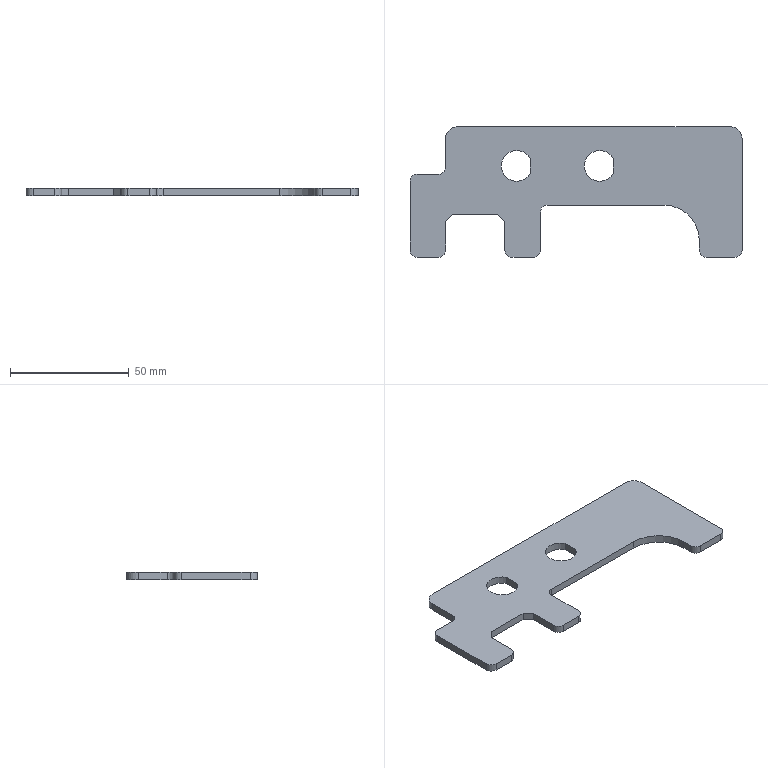Part | SolidWorks | features FlatPattern 1, SMBaseFlange 1, SheetMetal 1 | 1 solid | 36 faces | box 140 x 55 x 3.2 mm | volume 16813 mm3 | plane 20 | cylinder 16 | commonest cylinder face diameters 6 x9 13 x4 10 x2 30 x1
STEP:
#1=CARTESIAN_POINT('',(-66.3,99.624,3.2));
#2=VERTEX_POINT('',#1);
#3=CARTESIAN_POINT('',(-78.5,96.5,3.2));
#4=VERTEX_POINT('',#3);
#5=CARTESIAN_POINT('',(-72.,96.5,3.2));
#6=DIRECTION('',(0.,0.,1.));
#7=DIRECTION('',(1.,0.,0.));
#8=AXIS2_PLACEMENT_3D('',#5,#6,#7);
#9=CIRCLE('',#8,6.5);
#10=EDGE_CURVE('',#2,#4,#9,.T.);
#11=ORIENTED_EDGE('',*,*,#10,.T.);
#12=CARTESIAN_POINT('',(-78.5,96.5,0.));
#13=VERTEX_POINT('',#12);
#14=CARTESIAN_POINT('',(-78.5,96.5,3.2));
#15=DIRECTION('',(0.,0.,-1.));
#16=VECTOR('',#15,1000.);
#17=LINE('',#14,#16);
#18=EDGE_CURVE('',#4,#13,#17,.T.);
#19=ORIENTED_EDGE('',*,*,#18,.T.);
#20=CARTESIAN_POINT('',(-66.3,99.624,0.));
#21=VERTEX_POINT('',#20);
#22=CARTESIAN_POINT('',(-72.,96.5,0.));
#23=DIRECTION('',(0.,0.,1.));
#24=DIRECTION('',(1.,0.,0.));
#25=AXIS2_PLACEMENT_3D('',#22,#23,#24);
#26=CIRCLE('',#25,6.5);
#27=EDGE_CURVE('',#21,#13,#26,.T.);
#28=ORIENTED_EDGE('',*,*,#27,.F.);
#29=CARTESIAN_POINT('',(-66.3,99.624,3.2));
#30=DIRECTION('',(0.,0.,-1.));
#31=VECTOR('',#30,1000.);
#32=LINE('',#29,#31);
#33=EDGE_CURVE('',#2,#21,#32,.T.);
#34=ORIENTED_EDGE('',*,*,#33,.F.);
#35=EDGE_LOOP('',(#11,#19,#28,#34));
#36=FACE_OUTER_BOUND('',#35,.T.);
#37=CARTESIAN_POINT('',(-72.,96.5,3.2));
#38=DIRECTION('',(0.,0.,-1.));
#39=DIRECTION('',(-1.,0.,0.));
#40=AXIS2_PLACEMENT_3D('',#37,#38,#39);
#41=CYLINDRICAL_SURFACE('',#40,6.5);
#42=ADVANCED_FACE('',(#36),#41,.F.);
#43=CARTESIAN_POINT('',(-101.3,99.624,3.2));
#44=VERTEX_POINT('',#43);
#45=CARTESIAN_POINT('',(-113.5,96.5,3.2));
#46=VERTEX_POINT('',#45);
#47=CARTESIAN_POINT('',(-107.,96.5,3.2));
#48=DIRECTION('',(0.,0.,1.));
#49=DIRECTION('',(1.,0.,0.));
#50=AXIS2_PLACEMENT_3D('',#47,#48,#49);
#51=CIRCLE('',#50,6.5);
#52=EDGE_CURVE('',#44,#46,#51,.T.);
#53=ORIENTED_EDGE('',*,*,#52,.T.);
#54=CARTESIAN_POINT('',(-113.5,96.5,0.));
#55=VERTEX_POINT('',#54);
#56=CARTESIAN_POINT('',(-113.5,96.5,3.2));
#57=DIRECTION('',(0.,0.,-1.));
#58=VECTOR('',#57,1000.);
#59=LINE('',#56,#58);
#60=EDGE_CURVE('',#46,#55,#59,.T.);
#61=ORIENTED_EDGE('',*,*,#60,.T.);
#62=CARTESIAN_POINT('',(-101.3,99.624,0.));
#63=VERTEX_POINT('',#62);
#64=CARTESIAN_POINT('',(-107.,96.5,0.));
#65=DIRECTION('',(0.,0.,1.));
#66=DIRECTION('',(1.,0.,0.));
#67=AXIS2_PLACEMENT_3D('',#64,#65,#66);
#68=CIRCLE('',#67,6.5);
#69=EDGE_CURVE('',#63,#55,#68,.T.);
#70=ORIENTED_EDGE('',*,*,#69,.F.);
#71=CARTESIAN_POINT('',(-101.3,99.624,3.2));
#72=DIRECTION('',(0.,0.,-1.));
#73=VECTOR('',#72,1000.);
#74=LINE('',#71,#73);
#75=EDGE_CURVE('',#44,#63,#74,.T.);
#76=ORIENTED_EDGE('',*,*,#75,.F.);
#77=EDGE_LOOP('',(#53,#61,#70,#76));
#78=FACE_OUTER_BOUND('',#77,.T.);
#79=CARTESIAN_POINT('',(-107.,96.5,3.2));
#80=DIRECTION('',(0.,0.,-1.));
#81=DIRECTION('',(-1.,0.,0.));
#82=AXIS2_PLACEMENT_3D('',#79,#80,#81);
#83=CYLINDRICAL_SURFACE('',#82,6.5);
#84=ADVANCED_FACE('',(#78),#83,.F.);
#85=ORIENTED_EDGE('',*,*,#52,.F.);
#86=CARTESIAN_POINT('',(-101.3,93.376,3.2));
#87=VERTEX_POINT('',#86);
#88=CARTESIAN_POINT('',(-101.3,93.376,3.2));
#89=DIRECTION('',(0.,1.,0.));
#90=VECTOR('',#89,1000.);
#91=LINE('',#88,#90);
#92=EDGE_CURVE('',#87,#44,#91,.T.);
#93=ORIENTED_EDGE('',*,*,#92,.F.);
#94=CARTESIAN_POINT('',(-107.,96.5,3.2));
#95=DIRECTION('',(0.,0.,1.));
#96=DIRECTION('',(1.,0.,0.));
#97=AXIS2_PLACEMENT_3D('',#94,#95,#96);
#98=CIRCLE('',#97,6.5);
#99=EDGE_CURVE('',#46,#87,#98,.T.);
#100=ORIENTED_EDGE('',*,*,#99,.F.);
#101=EDGE_LOOP('',(#85,#93,#100));
#102=FACE_BOUND('',#101,.T.);
#103=CARTESIAN_POINT('',(-137.,96.,3.2));
#104=VERTEX_POINT('',#103);
#105=CARTESIAN_POINT('',(-140.,93.,3.2));
#106=VERTEX_POINT('',#105);
#107=CARTESIAN_POINT('',(-140.,96.,3.2));
#108=DIRECTION('',(0.,0.,-1.));
#109=DIRECTION('',(-1.,0.,0.));
#110=AXIS2_PLACEMENT_3D('',#107,#108,#109);
#111=CIRCLE('',#110,3.);
#112=EDGE_CURVE('',#104,#106,#111,.T.);
#113=ORIENTED_EDGE('',*,*,#112,.T.);
#114=CARTESIAN_POINT('',(-149.,93.,3.2));
#115=VERTEX_POINT('',#114);
#116=CARTESIAN_POINT('',(-140.,93.,3.2));
#117=DIRECTION('',(-1.,0.,0.));
#118=VECTOR('',#117,1000.);
#119=LINE('',#116,#118);
#120=EDGE_CURVE('',#106,#115,#119,.T.);
#121=ORIENTED_EDGE('',*,*,#120,.T.);
#122=CARTESIAN_POINT('',(-152.,90.,3.2));
#123=VERTEX_POINT('',#122);
#124=CARTESIAN_POINT('',(-149.,90.,3.2));
#125=DIRECTION('',(0.,0.,1.));
#126=DIRECTION('',(1.,0.,0.));
#127=AXIS2_PLACEMENT_3D('',#124,#125,#126);
#128=CIRCLE('',#127,3.);
#129=EDGE_CURVE('',#115,#123,#128,.T.);
#130=ORIENTED_EDGE('',*,*,#129,.T.);
#131=CARTESIAN_POINT('',(-152.,61.,3.2));
#132=VERTEX_POINT('',#131);
#133=CARTESIAN_POINT('',(-152.,90.,3.2));
#134=DIRECTION('',(0.,-1.,0.));
#135=VECTOR('',#134,1000.);
#136=LINE('',#133,#135);
#137=EDGE_CURVE('',#123,#132,#136,.T.);
#138=ORIENTED_EDGE('',*,*,#137,.T.);
#139=CARTESIAN_POINT('',(-149.,58.,3.2));
#140=VERTEX_POINT('',#139);
#141=CARTESIAN_POINT('',(-149.,61.,3.2));
#142=DIRECTION('',(0.,0.,1.));
#143=DIRECTION('',(1.,0.,0.));
#144=AXIS2_PLACEMENT_3D('',#141,#142,#143);
#145=CIRCLE('',#144,3.);
#146=EDGE_CURVE('',#132,#140,#145,.T.);
#147=ORIENTED_EDGE('',*,*,#146,.T.);
#148=CARTESIAN_POINT('',(-140.,58.,3.2));
#149=VERTEX_POINT('',#148);
#150=CARTESIAN_POINT('',(-149.,58.,3.2));
#151=DIRECTION('',(1.,0.,0.));
#152=VECTOR('',#151,1000.);
#153=LINE('',#150,#152);
#154=EDGE_CURVE('',#140,#149,#153,.T.);
#155=ORIENTED_EDGE('',*,*,#154,.T.);
#156=CARTESIAN_POINT('',(-137.,61.,3.2));
#157=VERTEX_POINT('',#156);
#158=CARTESIAN_POINT('',(-140.,61.,3.2));
#159=DIRECTION('',(0.,0.,1.));
#160=DIRECTION('',(1.,0.,0.));
#161=AXIS2_PLACEMENT_3D('',#158,#159,#160);
#162=CIRCLE('',#161,3.);
#163=EDGE_CURVE('',#149,#157,#162,.T.);
#164=ORIENTED_EDGE('',*,*,#163,.T.);
#165=CARTESIAN_POINT('',(-137.,73.,3.2));
#166=VERTEX_POINT('',#165);
#167=CARTESIAN_POINT('',(-137.,73.,3.2));
#168=DIRECTION('',(0.,1.,0.));
#169=VECTOR('',#168,1000.);
#170=LINE('',#167,#169);
#171=EDGE_CURVE('',#157,#166,#170,.T.);
#172=ORIENTED_EDGE('',*,*,#171,.T.);
#173=CARTESIAN_POINT('',(-134.,76.,3.2));
#174=VERTEX_POINT('',#173);
#175=CARTESIAN_POINT('',(-134.,76.,3.2));
#176=DIRECTION('',(0.7071,0.7071,0.));
#177=VECTOR('',#176,1000.);
#178=LINE('',#175,#177);
#179=EDGE_CURVE('',#166,#174,#178,.T.);
#180=ORIENTED_EDGE('',*,*,#179,.T.);
#181=CARTESIAN_POINT('',(-115.,76.,3.2));
#182=VERTEX_POINT('',#181);
#183=CARTESIAN_POINT('',(-115.,76.,3.2));
#184=DIRECTION('',(1.,0.,0.));
#185=VECTOR('',#184,1000.);
#186=LINE('',#183,#185);
#187=EDGE_CURVE('',#174,#182,#186,.T.);
#188=ORIENTED_EDGE('',*,*,#187,.T.);
#189=CARTESIAN_POINT('',(-112.,73.,3.2));
#190=VERTEX_POINT('',#189);
#191=CARTESIAN_POINT('',(-112.,73.,3.2));
#192=DIRECTION('',(0.7071,-0.7071,0.));
#193=VECTOR('',#192,1000.);
#194=LINE('',#191,#193);
#195=EDGE_CURVE('',#182,#190,#194,.T.);
#196=ORIENTED_EDGE('',*,*,#195,.T.);
#197=CARTESIAN_POINT('',(-112.,61.,3.2));
#198=VERTEX_POINT('',#197);
#199=CARTESIAN_POINT('',(-112.,61.,3.2));
#200=DIRECTION('',(0.,-1.,0.));
#201=VECTOR('',#200,1000.);
#202=LINE('',#199,#201);
#203=EDGE_CURVE('',#190,#198,#202,.T.);
#204=ORIENTED_EDGE('',*,*,#203,.T.);
#205=CARTESIAN_POINT('',(-109.,58.,3.2));
#206=VERTEX_POINT('',#205);
#207=CARTESIAN_POINT('',(-109.,61.,3.2));
#208=DIRECTION('',(0.,0.,1.));
#209=DIRECTION('',(-1.,0.,0.));
#210=AXIS2_PLACEMENT_3D('',#207,#208,#209);
#211=CIRCLE('',#210,3.);
#212=EDGE_CURVE('',#198,#206,#211,.T.);
#213=ORIENTED_EDGE('',*,*,#212,.T.);
#214=CARTESIAN_POINT('',(-100.,58.,3.2));
#215=VERTEX_POINT('',#214);
#216=CARTESIAN_POINT('',(-100.,58.,3.2));
#217=DIRECTION('',(1.,0.,0.));
#218=VECTOR('',#217,1000.);
#219=LINE('',#216,#218);
#220=EDGE_CURVE('',#206,#215,#219,.T.);
#221=ORIENTED_EDGE('',*,*,#220,.T.);
#222=CARTESIAN_POINT('',(-97.,61.,3.2));
#223=VERTEX_POINT('',#222);
#224=CARTESIAN_POINT('',(-100.,61.,3.2));
#225=DIRECTION('',(0.,0.,1.));
#226=DIRECTION('',(-1.,0.,0.));
#227=AXIS2_PLACEMENT_3D('',#224,#225,#226);
#228=CIRCLE('',#227,3.);
#229=EDGE_CURVE('',#215,#223,#228,.T.);
#230=ORIENTED_EDGE('',*,*,#229,.T.);
#231=CARTESIAN_POINT('',(-97.,77.,3.2));
#232=VERTEX_POINT('',#231);
#233=CARTESIAN_POINT('',(-97.,77.,3.2));
#234=DIRECTION('',(0.,1.,0.));
#235=VECTOR('',#234,1000.);
#236=LINE('',#233,#235);
#237=EDGE_CURVE('',#223,#232,#236,.T.);
#238=ORIENTED_EDGE('',*,*,#237,.T.);
#239=CARTESIAN_POINT('',(-94.,80.,3.2));
#240=VERTEX_POINT('',#239);
#241=CARTESIAN_POINT('',(-94.,77.,3.2));
#242=DIRECTION('',(0.,0.,-1.));
#243=DIRECTION('',(1.,0.,0.));
#244=AXIS2_PLACEMENT_3D('',#241,#242,#243);
#245=CIRCLE('',#244,3.);
#246=EDGE_CURVE('',#232,#240,#245,.T.);
#247=ORIENTED_EDGE('',*,*,#246,.T.);
#248=CARTESIAN_POINT('',(-45.,80.,3.2));
#249=VERTEX_POINT('',#248);
#250=CARTESIAN_POINT('',(-94.,80.,3.2));
#251=DIRECTION('',(1.,0.,0.));
#252=VECTOR('',#251,1000.);
#253=LINE('',#250,#252);
#254=EDGE_CURVE('',#240,#249,#253,.T.);
#255=ORIENTED_EDGE('',*,*,#254,.T.);
#256=CARTESIAN_POINT('',(-30.,65.,3.2));
#257=VERTEX_POINT('',#256);
#258=CARTESIAN_POINT('',(-45.,65.,3.2));
#259=DIRECTION('',(0.,0.,-1.));
#260=DIRECTION('',(-1.,0.,0.));
#261=AXIS2_PLACEMENT_3D('',#258,#259,#260);
#262=CIRCLE('',#261,15.);
#263=EDGE_CURVE('',#249,#257,#262,.T.);
#264=ORIENTED_EDGE('',*,*,#263,.T.);
#265=CARTESIAN_POINT('',(-30.,61.,3.2));
#266=VERTEX_POINT('',#265);
#267=CARTESIAN_POINT('',(-30.,61.,3.2));
#268=DIRECTION('',(0.,-1.,0.));
#269=VECTOR('',#268,1000.);
#270=LINE('',#267,#269);
#271=EDGE_CURVE('',#257,#266,#270,.T.);
#272=ORIENTED_EDGE('',*,*,#271,.T.);
#273=CARTESIAN_POINT('',(-27.,58.,3.2));
#274=VERTEX_POINT('',#273);
#275=CARTESIAN_POINT('',(-27.,61.,3.2));
#276=DIRECTION('',(0.,0.,1.));
#277=DIRECTION('',(-1.,0.,0.));
#278=AXIS2_PLACEMENT_3D('',#275,#276,#277);
#279=CIRCLE('',#278,3.);
#280=EDGE_CURVE('',#266,#274,#279,.T.);
#281=ORIENTED_EDGE('',*,*,#280,.T.);
#282=CARTESIAN_POINT('',(-15.,58.,3.2));
#283=VERTEX_POINT('',#282);
#284=CARTESIAN_POINT('',(-15.,58.,3.2));
#285=DIRECTION('',(1.,0.,0.));
#286=VECTOR('',#285,1000.);
#287=LINE('',#284,#286);
#288=EDGE_CURVE('',#274,#283,#287,.T.);
#289=ORIENTED_EDGE('',*,*,#288,.T.);
#290=CARTESIAN_POINT('',(-12.,61.,3.2));
#291=VERTEX_POINT('',#290);
#292=CARTESIAN_POINT('',(-15.,61.,3.2));
#293=DIRECTION('',(0.,0.,1.));
#294=DIRECTION('',(-1.,0.,0.));
#295=AXIS2_PLACEMENT_3D('',#292,#293,#294);
#296=CIRCLE('',#295,3.);
#297=EDGE_CURVE('',#283,#291,#296,.T.);
#298=ORIENTED_EDGE('',*,*,#297,.T.);
#299=CARTESIAN_POINT('',(-12.,108.,3.2));
#300=VERTEX_POINT('',#299);
#301=CARTESIAN_POINT('',(-12.,108.,3.2));
#302=DIRECTION('',(0.,1.,0.));
#303=VECTOR('',#302,1000.);
#304=LINE('',#301,#303);
#305=EDGE_CURVE('',#291,#300,#304,.T.);
#306=ORIENTED_EDGE('',*,*,#305,.T.);
#307=CARTESIAN_POINT('',(-17.,113.,3.2));
#308=VERTEX_POINT('',#307);
#309=CARTESIAN_POINT('',(-17.,108.,3.2));
#310=DIRECTION('',(0.,0.,1.));
#311=DIRECTION('',(1.,0.,0.));
#312=AXIS2_PLACEMENT_3D('',#309,#310,#311);
#313=CIRCLE('',#312,5.);
#314=EDGE_CURVE('',#300,#308,#313,.T.);
#315=ORIENTED_EDGE('',*,*,#314,.T.);
#316=CARTESIAN_POINT('',(-132.,113.,3.2));
#317=VERTEX_POINT('',#316);
#318=CARTESIAN_POINT('',(-17.,113.,3.2));
#319=DIRECTION('',(-1.,0.,0.));
#320=VECTOR('',#319,1000.);
#321=LINE('',#318,#320);
#322=EDGE_CURVE('',#308,#317,#321,.T.);
#323=ORIENTED_EDGE('',*,*,#322,.T.);
#324=CARTESIAN_POINT('',(-137.,108.,3.2));
#325=VERTEX_POINT('',#324);
#326=CARTESIAN_POINT('',(-132.,108.,3.2));
#327=DIRECTION('',(0.,0.,1.));
#328=DIRECTION('',(-1.,0.,0.));
#329=AXIS2_PLACEMENT_3D('',#326,#327,#328);
#330=CIRCLE('',#329,5.);
#331=EDGE_CURVE('',#317,#325,#330,.T.);
#332=ORIENTED_EDGE('',*,*,#331,.T.);
#333=CARTESIAN_POINT('',(-137.,108.,3.2));
#334=DIRECTION('',(0.,-1.,0.));
#335=VECTOR('',#334,1000.);
#336=LINE('',#333,#335);
#337=EDGE_CURVE('',#325,#104,#336,.T.);
#338=ORIENTED_EDGE('',*,*,#337,.T.);
#339=EDGE_LOOP('',(#113,#121,#130,#138,#147,#155,#164,#172,#180,#188,#196,#204,#213,#221,#230,#238,#247,#255,#264,#272,#281,#289,#298,#306,#315,#323,#332,#338));
#340=FACE_OUTER_BOUND('',#339,.T.);
#341=ORIENTED_EDGE('',*,*,#10,.F.);
#342=CARTESIAN_POINT('',(-66.3,93.376,3.2));
#343=VERTEX_POINT('',#342);
#344=CARTESIAN_POINT('',(-66.3,93.376,3.2));
#345=DIRECTION('',(0.,1.,0.));
#346=VECTOR('',#345,1000.);
#347=LINE('',#344,#346);
#348=EDGE_CURVE('',#343,#2,#347,.T.);
#349=ORIENTED_EDGE('',*,*,#348,.F.);
#350=CARTESIAN_POINT('',(-72.,96.5,3.2));
#351=DIRECTION('',(0.,0.,1.));
#352=DIRECTION('',(1.,0.,0.));
#353=AXIS2_PLACEMENT_3D('',#350,#351,#352);
#354=CIRCLE('',#353,6.5);
#355=EDGE_CURVE('',#4,#343,#354,.T.);
#356=ORIENTED_EDGE('',*,*,#355,.F.);
#357=EDGE_LOOP('',(#341,#349,#356));
#358=FACE_BOUND('',#357,.T.);
#359=CARTESIAN_POINT('',(-140.,96.,3.2));
#360=DIRECTION('',(0.,0.,-1.));
#361=DIRECTION('',(-1.,0.,0.));
#362=AXIS2_PLACEMENT_3D('',#359,#360,#361);
#363=PLANE('',#362);
#364=ADVANCED_FACE('',(#102,#340,#358),#363,.F.);
#365=CARTESIAN_POINT('',(-137.,96.,0.));
#366=VERTEX_POINT('',#365);
#367=CARTESIAN_POINT('',(-140.,93.,0.));
#368=VERTEX_POINT('',#367);
#369=CARTESIAN_POINT('',(-140.,96.,0.));
#370=DIRECTION('',(0.,0.,-1.));
#371=DIRECTION('',(-1.,0.,0.));
#372=AXIS2_PLACEMENT_3D('',#369,#370,#371);
#373=CIRCLE('',#372,3.);
#374=EDGE_CURVE('',#366,#368,#373,.T.);
#375=ORIENTED_EDGE('',*,*,#374,.F.);
#376=CARTESIAN_POINT('',(-137.,108.,0.));
#377=VERTEX_POINT('',#376);
#378=CARTESIAN_POINT('',(-137.,108.,0.));
#379=DIRECTION('',(0.,-1.,0.));
#380=VECTOR('',#379,1000.);
#381=LINE('',#378,#380);
#382=EDGE_CURVE('',#377,#366,#381,.T.);
#383=ORIENTED_EDGE('',*,*,#382,.F.);
#384=CARTESIAN_POINT('',(-132.,113.,0.));
#385=VERTEX_POINT('',#384);
#386=CARTESIAN_POINT('',(-132.,108.,0.));
#387=DIRECTION('',(0.,0.,1.));
#388=DIRECTION('',(-1.,0.,0.));
#389=AXIS2_PLACEMENT_3D('',#386,#387,#388);
#390=CIRCLE('',#389,5.);
#391=EDGE_CURVE('',#385,#377,#390,.T.);
#392=ORIENTED_EDGE('',*,*,#391,.F.);
#393=CARTESIAN_POINT('',(-17.,113.,0.));
#394=VERTEX_POINT('',#393);
#395=CARTESIAN_POINT('',(-17.,113.,0.));
#396=DIRECTION('',(-1.,0.,0.));
#397=VECTOR('',#396,1000.);
#398=LINE('',#395,#397);
#399=EDGE_CURVE('',#394,#385,#398,.T.);
#400=ORIENTED_EDGE('',*,*,#399,.F.);
#401=CARTESIAN_POINT('',(-12.,108.,0.));
#402=VERTEX_POINT('',#401);
#403=CARTESIAN_POINT('',(-17.,108.,0.));
#404=DIRECTION('',(0.,0.,1.));
#405=DIRECTION('',(1.,0.,0.));
#406=AXIS2_PLACEMENT_3D('',#403,#404,#405);
#407=CIRCLE('',#406,5.);
#408=EDGE_CURVE('',#402,#394,#407,.T.);
#409=ORIENTED_EDGE('',*,*,#408,.F.);
#410=CARTESIAN_POINT('',(-12.,61.,0.));
#411=VERTEX_POINT('',#410);
#412=CARTESIAN_POINT('',(-12.,108.,0.));
#413=DIRECTION('',(0.,1.,0.));
#414=VECTOR('',#413,1000.);
#415=LINE('',#412,#414);
#416=EDGE_CURVE('',#411,#402,#415,.T.);
#417=ORIENTED_EDGE('',*,*,#416,.F.);
#418=CARTESIAN_POINT('',(-15.,58.,0.));
#419=VERTEX_POINT('',#418);
#420=CARTESIAN_POINT('',(-15.,61.,0.));
#421=DIRECTION('',(0.,0.,1.));
#422=DIRECTION('',(-1.,0.,0.));
#423=AXIS2_PLACEMENT_3D('',#420,#421,#422);
#424=CIRCLE('',#423,3.);
#425=EDGE_CURVE('',#419,#411,#424,.T.);
#426=ORIENTED_EDGE('',*,*,#425,.F.);
#427=CARTESIAN_POINT('',(-27.,58.,0.));
#428=VERTEX_POINT('',#427);
#429=CARTESIAN_POINT('',(-15.,58.,0.));
#430=DIRECTION('',(1.,0.,0.));
#431=VECTOR('',#430,1000.);
#432=LINE('',#429,#431);
#433=EDGE_CURVE('',#428,#419,#432,.T.);
#434=ORIENTED_EDGE('',*,*,#433,.F.);
#435=CARTESIAN_POINT('',(-30.,61.,0.));
#436=VERTEX_POINT('',#435);
#437=CARTESIAN_POINT('',(-27.,61.,0.));
#438=DIRECTION('',(0.,0.,1.));
#439=DIRECTION('',(-1.,0.,0.));
#440=AXIS2_PLACEMENT_3D('',#437,#438,#439);
#441=CIRCLE('',#440,3.);
#442=EDGE_CURVE('',#436,#428,#441,.T.);
#443=ORIENTED_EDGE('',*,*,#442,.F.);
#444=CARTESIAN_POINT('',(-30.,65.,0.));
#445=VERTEX_POINT('',#444);
#446=CARTESIAN_POINT('',(-30.,61.,0.));
#447=DIRECTION('',(0.,-1.,0.));
#448=VECTOR('',#447,1000.);
#449=LINE('',#446,#448);
#450=EDGE_CURVE('',#445,#436,#449,.T.);
#451=ORIENTED_EDGE('',*,*,#450,.F.);
#452=CARTESIAN_POINT('',(-45.,80.,0.));
#453=VERTEX_POINT('',#452);
#454=CARTESIAN_POINT('',(-45.,65.,0.));
#455=DIRECTION('',(0.,0.,-1.));
#456=DIRECTION('',(-1.,0.,0.));
#457=AXIS2_PLACEMENT_3D('',#454,#455,#456);
#458=CIRCLE('',#457,15.);
#459=EDGE_CURVE('',#453,#445,#458,.T.);
#460=ORIENTED_EDGE('',*,*,#459,.F.);
#461=CARTESIAN_POINT('',(-94.,80.,0.));
#462=VERTEX_POINT('',#461);
#463=CARTESIAN_POINT('',(-94.,80.,0.));
#464=DIRECTION('',(1.,0.,0.));
#465=VECTOR('',#464,1000.);
#466=LINE('',#463,#465);
#467=EDGE_CURVE('',#462,#453,#466,.T.);
#468=ORIENTED_EDGE('',*,*,#467,.F.);
#469=CARTESIAN_POINT('',(-97.,77.,0.));
#470=VERTEX_POINT('',#469);
#471=CARTESIAN_POINT('',(-94.,77.,0.));
#472=DIRECTION('',(0.,0.,-1.));
#473=DIRECTION('',(1.,0.,0.));
#474=AXIS2_PLACEMENT_3D('',#471,#472,#473);
#475=CIRCLE('',#474,3.);
#476=EDGE_CURVE('',#470,#462,#475,.T.);
#477=ORIENTED_EDGE('',*,*,#476,.F.);
#478=CARTESIAN_POINT('',(-97.,61.,0.));
#479=VERTEX_POINT('',#478);
#480=CARTESIAN_POINT('',(-97.,77.,0.));
#481=DIRECTION('',(0.,1.,0.));
#482=VECTOR('',#481,1000.);
#483=LINE('',#480,#482);
#484=EDGE_CURVE('',#479,#470,#483,.T.);
#485=ORIENTED_EDGE('',*,*,#484,.F.);
#486=CARTESIAN_POINT('',(-100.,58.,0.));
#487=VERTEX_POINT('',#486);
#488=CARTESIAN_POINT('',(-100.,61.,0.));
#489=DIRECTION('',(0.,0.,1.));
#490=DIRECTION('',(-1.,0.,0.));
#491=AXIS2_PLACEMENT_3D('',#488,#489,#490);
#492=CIRCLE('',#491,3.);
#493=EDGE_CURVE('',#487,#479,#492,.T.);
#494=ORIENTED_EDGE('',*,*,#493,.F.);
#495=CARTESIAN_POINT('',(-109.,58.,0.));
#496=VERTEX_POINT('',#495);
#497=CARTESIAN_POINT('',(-100.,58.,0.));
#498=DIRECTION('',(1.,0.,0.));
#499=VECTOR('',#498,1000.);
#500=LINE('',#497,#499);
#501=EDGE_CURVE('',#496,#487,#500,.T.);
#502=ORIENTED_EDGE('',*,*,#501,.F.);
#503=CARTESIAN_POINT('',(-112.,61.,0.));
#504=VERTEX_POINT('',#503);
#505=CARTESIAN_POINT('',(-109.,61.,0.));
#506=DIRECTION('',(0.,0.,1.));
#507=DIRECTION('',(-1.,0.,0.));
#508=AXIS2_PLACEMENT_3D('',#505,#506,#507);
#509=CIRCLE('',#508,3.);
#510=EDGE_CURVE('',#504,#496,#509,.T.);
#511=ORIENTED_EDGE('',*,*,#510,.F.);
#512=CARTESIAN_POINT('',(-112.,73.,0.));
#513=VERTEX_POINT('',#512);
#514=CARTESIAN_POINT('',(-112.,61.,0.));
#515=DIRECTION('',(0.,-1.,0.));
#516=VECTOR('',#515,1000.);
#517=LINE('',#514,#516);
#518=EDGE_CURVE('',#513,#504,#517,.T.);
#519=ORIENTED_EDGE('',*,*,#518,.F.);
#520=CARTESIAN_POINT('',(-115.,76.,0.));
#521=VERTEX_POINT('',#520);
#522=CARTESIAN_POINT('',(-112.,73.,0.));
#523=DIRECTION('',(0.7071,-0.7071,0.));
#524=VECTOR('',#523,1000.);
#525=LINE('',#522,#524);
#526=EDGE_CURVE('',#521,#513,#525,.T.);
#527=ORIENTED_EDGE('',*,*,#526,.F.);
#528=CARTESIAN_POINT('',(-134.,76.,0.));
#529=VERTEX_POINT('',#528);
#530=CARTESIAN_POINT('',(-115.,76.,0.));
#531=DIRECTION('',(1.,0.,0.));
#532=VECTOR('',#531,1000.);
#533=LINE('',#530,#532);
#534=EDGE_CURVE('',#529,#521,#533,.T.);
#535=ORIENTED_EDGE('',*,*,#534,.F.);
#536=CARTESIAN_POINT('',(-137.,73.,0.));
#537=VERTEX_POINT('',#536);
#538=CARTESIAN_POINT('',(-134.,76.,0.));
#539=DIRECTION('',(0.7071,0.7071,0.));
#540=VECTOR('',#539,1000.);
#541=LINE('',#538,#540);
#542=EDGE_CURVE('',#537,#529,#541,.T.);
#543=ORIENTED_EDGE('',*,*,#542,.F.);
#544=CARTESIAN_POINT('',(-137.,61.,0.));
#545=VERTEX_POINT('',#544);
#546=CARTESIAN_POINT('',(-137.,73.,0.));
#547=DIRECTION('',(0.,1.,0.));
#548=VECTOR('',#547,1000.);
#549=LINE('',#546,#548);
#550=EDGE_CURVE('',#545,#537,#549,.T.);
#551=ORIENTED_EDGE('',*,*,#550,.F.);
#552=CARTESIAN_POINT('',(-140.,58.,0.));
#553=VERTEX_POINT('',#552);
#554=CARTESIAN_POINT('',(-140.,61.,0.));
#555=DIRECTION('',(0.,0.,1.));
#556=DIRECTION('',(1.,0.,0.));
#557=AXIS2_PLACEMENT_3D('',#554,#555,#556);
#558=CIRCLE('',#557,3.);
#559=EDGE_CURVE('',#553,#545,#558,.T.);
#560=ORIENTED_EDGE('',*,*,#559,.F.);
#561=CARTESIAN_POINT('',(-149.,58.,0.));
#562=VERTEX_POINT('',#561);
#563=CARTESIAN_POINT('',(-149.,58.,0.));
#564=DIRECTION('',(1.,0.,0.));
#565=VECTOR('',#564,1000.);
#566=LINE('',#563,#565);
#567=EDGE_CURVE('',#562,#553,#566,.T.);
#568=ORIENTED_EDGE('',*,*,#567,.F.);
#569=CARTESIAN_POINT('',(-152.,61.,0.));
#570=VERTEX_POINT('',#569);
#571=CARTESIAN_POINT('',(-149.,61.,0.));
#572=DIRECTION('',(0.,0.,1.));
#573=DIRECTION('',(1.,0.,0.));
#574=AXIS2_PLACEMENT_3D('',#571,#572,#573);
#575=CIRCLE('',#574,3.);
#576=EDGE_CURVE('',#570,#562,#575,.T.);
#577=ORIENTED_EDGE('',*,*,#576,.F.);
#578=CARTESIAN_POINT('',(-152.,90.,0.));
#579=VERTEX_POINT('',#578);
#580=CARTESIAN_POINT('',(-152.,90.,0.));
#581=DIRECTION('',(0.,-1.,0.));
#582=VECTOR('',#581,1000.);
#583=LINE('',#580,#582);
#584=EDGE_CURVE('',#579,#570,#583,.T.);
#585=ORIENTED_EDGE('',*,*,#584,.F.);
#586=CARTESIAN_POINT('',(-149.,93.,0.));
#587=VERTEX_POINT('',#586);
#588=CARTESIAN_POINT('',(-149.,90.,0.));
#589=DIRECTION('',(0.,0.,1.));
#590=DIRECTION('',(1.,0.,0.));
#591=AXIS2_PLACEMENT_3D('',#588,#589,#590);
#592=CIRCLE('',#591,3.);
#593=EDGE_CURVE('',#587,#579,#592,.T.);
#594=ORIENTED_EDGE('',*,*,#593,.F.);
#595=CARTESIAN_POINT('',(-140.,93.,0.));
#596=DIRECTION('',(-1.,0.,0.));
#597=VECTOR('',#596,1000.);
#598=LINE('',#595,#597);
#599=EDGE_CURVE('',#368,#587,#598,.T.);
#600=ORIENTED_EDGE('',*,*,#599,.F.);
#601=EDGE_LOOP('',(#375,#383,#392,#400,#409,#417,#426,#434,#443,#451,#460,#468,#477,#485,#494,#502,#511,#519,#527,#535,#543,#551,#560,#568,#577,#585,#594,#600));
#602=FACE_OUTER_BOUND('',#601,.T.);
#603=CARTESIAN_POINT('',(-101.3,93.376,0.));
#604=VERTEX_POINT('',#603);
#605=CARTESIAN_POINT('',(-101.3,93.376,0.));
#606=DIRECTION('',(0.,1.,0.));
#607=VECTOR('',#606,1000.);
#608=LINE('',#605,#607);
#609=EDGE_CURVE('',#604,#63,#608,.T.);
#610=ORIENTED_EDGE('',*,*,#609,.T.);
#611=ORIENTED_EDGE('',*,*,#69,.T.);
#612=CARTESIAN_POINT('',(-107.,96.5,0.));
#613=DIRECTION('',(0.,0.,1.));
#614=DIRECTION('',(1.,0.,0.));
#615=AXIS2_PLACEMENT_3D('',#612,#613,#614);
#616=CIRCLE('',#615,6.5);
#617=EDGE_CURVE('',#55,#604,#616,.T.);
#618=ORIENTED_EDGE('',*,*,#617,.T.);
#619=EDGE_LOOP('',(#610,#611,#618));
#620=FACE_BOUND('',#619,.T.);
#621=CARTESIAN_POINT('',(-66.3,93.376,0.));
#622=VERTEX_POINT('',#621);
#623=CARTESIAN_POINT('',(-66.3,93.376,0.));
#624=DIRECTION('',(0.,1.,0.));
#625=VECTOR('',#624,1000.);
#626=LINE('',#623,#625);
#627=EDGE_CURVE('',#622,#21,#626,.T.);
#628=ORIENTED_EDGE('',*,*,#627,.T.);
#629=ORIENTED_EDGE('',*,*,#27,.T.);
#630=CARTESIAN_POINT('',(-72.,96.5,0.));
#631=DIRECTION('',(0.,0.,1.));
#632=DIRECTION('',(1.,0.,0.));
#633=AXIS2_PLACEMENT_3D('',#630,#631,#632);
#634=CIRCLE('',#633,6.5);
#635=EDGE_CURVE('',#13,#622,#634,.T.);
#636=ORIENTED_EDGE('',*,*,#635,.T.);
#637=EDGE_LOOP('',(#628,#629,#636));
#638=FACE_BOUND('',#637,.T.);
#639=CARTESIAN_POINT('',(-140.,96.,0.));
#640=DIRECTION('',(0.,0.,-1.));
#641=DIRECTION('',(-1.,0.,0.));
#642=AXIS2_PLACEMENT_3D('',#639,#640,#641);
#643=PLANE('',#642);
#644=ADVANCED_FACE('',(#602,#620,#638),#643,.T.);
#645=ORIENTED_EDGE('',*,*,#374,.T.);
#646=CARTESIAN_POINT('',(-140.,93.,3.2));
#647=DIRECTION('',(0.,0.,-1.));
#648=VECTOR('',#647,1000.);
#649=LINE('',#646,#648);
#650=EDGE_CURVE('',#106,#368,#649,.T.);
#651=ORIENTED_EDGE('',*,*,#650,.F.);
#652=ORIENTED_EDGE('',*,*,#112,.F.);
#653=CARTESIAN_POINT('',(-137.,96.,3.2));
#654=DIRECTION('',(0.,0.,-1.));
#655=VECTOR('',#654,1000.);
#656=LINE('',#653,#655);
#657=EDGE_CURVE('',#104,#366,#656,.T.);
#658=ORIENTED_EDGE('',*,*,#657,.T.);
#659=EDGE_LOOP('',(#645,#651,#652,#658));
#660=FACE_OUTER_BOUND('',#659,.T.);
#661=CARTESIAN_POINT('',(-140.,96.,3.2));
#662=DIRECTION('',(0.,0.,-1.));
#663=DIRECTION('',(-1.,0.,0.));
#664=AXIS2_PLACEMENT_3D('',#661,#662,#663);
#665=CYLINDRICAL_SURFACE('',#664,3.);
#666=ADVANCED_FACE('',(#660),#665,.F.);
#667=ORIENTED_EDGE('',*,*,#599,.T.);
#668=CARTESIAN_POINT('',(-149.,93.,3.2));
#669=DIRECTION('',(0.,0.,-1.));
#670=VECTOR('',#669,1000.);
#671=LINE('',#668,#670);
#672=EDGE_CURVE('',#115,#587,#671,.T.);
#673=ORIENTED_EDGE('',*,*,#672,.F.);
#674=ORIENTED_EDGE('',*,*,#120,.F.);
#675=ORIENTED_EDGE('',*,*,#650,.T.);
#676=EDGE_LOOP('',(#667,#673,#674,#675));
#677=FACE_OUTER_BOUND('',#676,.T.);
#678=CARTESIAN_POINT('',(-140.,93.,3.2));
#679=DIRECTION('',(0.,-1.,0.));
#680=DIRECTION('',(0.,0.,-1.));
#681=AXIS2_PLACEMENT_3D('',#678,#679,#680);
#682=PLANE('',#681);
#683=ADVANCED_FACE('',(#677),#682,.F.);
#684=ORIENTED_EDGE('',*,*,#593,.T.);
#685=CARTESIAN_POINT('',(-152.,90.,3.2));
#686=DIRECTION('',(0.,0.,-1.));
#687=VECTOR('',#686,1000.);
#688=LINE('',#685,#687);
#689=EDGE_CURVE('',#123,#579,#688,.T.);
#690=ORIENTED_EDGE('',*,*,#689,.F.);
#691=ORIENTED_EDGE('',*,*,#129,.F.);
#692=ORIENTED_EDGE('',*,*,#672,.T.);
#693=EDGE_LOOP('',(#684,#690,#691,#692));
#694=FACE_OUTER_BOUND('',#693,.T.);
#695=CARTESIAN_POINT('',(-149.,90.,3.2));
#696=DIRECTION('',(0.,0.,-1.));
#697=DIRECTION('',(-1.,0.,0.));
#698=AXIS2_PLACEMENT_3D('',#695,#696,#697);
#699=CYLINDRICAL_SURFACE('',#698,3.);
#700=ADVANCED_FACE('',(#694),#699,.T.);
#701=ORIENTED_EDGE('',*,*,#584,.T.);
#702=CARTESIAN_POINT('',(-152.,61.,3.2));
#703=DIRECTION('',(0.,0.,-1.));
#704=VECTOR('',#703,1000.);
#705=LINE('',#702,#704);
#706=EDGE_CURVE('',#132,#570,#705,.T.);
#707=ORIENTED_EDGE('',*,*,#706,.F.);
#708=ORIENTED_EDGE('',*,*,#137,.F.);
#709=ORIENTED_EDGE('',*,*,#689,.T.);
#710=EDGE_LOOP('',(#701,#707,#708,#709));
#711=FACE_OUTER_BOUND('',#710,.T.);
#712=CARTESIAN_POINT('',(-152.,90.,3.2));
#713=DIRECTION('',(1.,0.,0.));
#714=DIRECTION('',(0.,0.,-1.));
#715=AXIS2_PLACEMENT_3D('',#712,#713,#714);
#716=PLANE('',#715);
#717=ADVANCED_FACE('',(#711),#716,.F.);
#718=ORIENTED_EDGE('',*,*,#576,.T.);
#719=CARTESIAN_POINT('',(-149.,58.,3.2));
#720=DIRECTION('',(0.,0.,-1.));
#721=VECTOR('',#720,1000.);
#722=LINE('',#719,#721);
#723=EDGE_CURVE('',#140,#562,#722,.T.);
#724=ORIENTED_EDGE('',*,*,#723,.F.);
#725=ORIENTED_EDGE('',*,*,#146,.F.);
#726=ORIENTED_EDGE('',*,*,#706,.T.);
#727=EDGE_LOOP('',(#718,#724,#725,#726));
#728=FACE_OUTER_BOUND('',#727,.T.);
#729=CARTESIAN_POINT('',(-149.,61.,3.2));
#730=DIRECTION('',(0.,0.,-1.));
#731=DIRECTION('',(-1.,0.,0.));
#732=AXIS2_PLACEMENT_3D('',#729,#730,#731);
#733=CYLINDRICAL_SURFACE('',#732,3.);
#734=ADVANCED_FACE('',(#728),#733,.T.);
#735=ORIENTED_EDGE('',*,*,#567,.T.);
#736=CARTESIAN_POINT('',(-140.,58.,3.2));
#737=DIRECTION('',(0.,0.,-1.));
#738=VECTOR('',#737,1000.);
#739=LINE('',#736,#738);
#740=EDGE_CURVE('',#149,#553,#739,.T.);
#741=ORIENTED_EDGE('',*,*,#740,.F.);
#742=ORIENTED_EDGE('',*,*,#154,.F.);
#743=ORIENTED_EDGE('',*,*,#723,.T.);
#744=EDGE_LOOP('',(#735,#741,#742,#743));
#745=FACE_OUTER_BOUND('',#744,.T.);
#746=CARTESIAN_POINT('',(-149.,58.,3.2));
#747=DIRECTION('',(0.,1.,0.));
#748=DIRECTION('',(0.,0.,1.));
#749=AXIS2_PLACEMENT_3D('',#746,#747,#748);
#750=PLANE('',#749);
#751=ADVANCED_FACE('',(#745),#750,.F.);
#752=ORIENTED_EDGE('',*,*,#559,.T.);
#753=CARTESIAN_POINT('',(-137.,61.,3.2));
#754=DIRECTION('',(0.,0.,-1.));
#755=VECTOR('',#754,1000.);
#756=LINE('',#753,#755);
#757=EDGE_CURVE('',#157,#545,#756,.T.);
#758=ORIENTED_EDGE('',*,*,#757,.F.);
#759=ORIENTED_EDGE('',*,*,#163,.F.);
#760=ORIENTED_EDGE('',*,*,#740,.T.);
#761=EDGE_LOOP('',(#752,#758,#759,#760));
#762=FACE_OUTER_BOUND('',#761,.T.);
#763=CARTESIAN_POINT('',(-140.,61.,3.2));
#764=DIRECTION('',(0.,0.,-1.));
#765=DIRECTION('',(-1.,0.,0.));
#766=AXIS2_PLACEMENT_3D('',#763,#764,#765);
#767=CYLINDRICAL_SURFACE('',#766,3.);
#768=ADVANCED_FACE('',(#762),#767,.T.);
#769=ORIENTED_EDGE('',*,*,#550,.T.);
#770=CARTESIAN_POINT('',(-137.,73.,3.2));
#771=DIRECTION('',(0.,0.,-1.));
#772=VECTOR('',#771,1000.);
#773=LINE('',#770,#772);
#774=EDGE_CURVE('',#166,#537,#773,.T.);
#775=ORIENTED_EDGE('',*,*,#774,.F.);
#776=ORIENTED_EDGE('',*,*,#171,.F.);
#777=ORIENTED_EDGE('',*,*,#757,.T.);
#778=EDGE_LOOP('',(#769,#775,#776,#777));
#779=FACE_OUTER_BOUND('',#778,.T.);
#780=CARTESIAN_POINT('',(-137.,73.,3.2));
#781=DIRECTION('',(-1.,0.,0.));
#782=DIRECTION('',(0.,-1.,0.));
#783=AXIS2_PLACEMENT_3D('',#780,#781,#782);
#784=PLANE('',#783);
#785=ADVANCED_FACE('',(#779),#784,.F.);
#786=ORIENTED_EDGE('',*,*,#542,.T.);
#787=CARTESIAN_POINT('',(-134.,76.,3.2));
#788=DIRECTION('',(0.,0.,-1.));
#789=VECTOR('',#788,1000.);
#790=LINE('',#787,#789);
#791=EDGE_CURVE('',#174,#529,#790,.T.);
#792=ORIENTED_EDGE('',*,*,#791,.F.);
#793=ORIENTED_EDGE('',*,*,#179,.F.);
#794=ORIENTED_EDGE('',*,*,#774,.T.);
#795=EDGE_LOOP('',(#786,#792,#793,#794));
#796=FACE_OUTER_BOUND('',#795,.T.);
#797=CARTESIAN_POINT('',(-134.,76.,3.2));
#798=DIRECTION('',(-0.7071,0.7071,0.));
#799=DIRECTION('',(-0.7071,-0.7071,0.));
#800=AXIS2_PLACEMENT_3D('',#797,#798,#799);
#801=PLANE('',#800);
#802=ADVANCED_FACE('',(#796),#801,.F.);
#803=ORIENTED_EDGE('',*,*,#534,.T.);
#804=CARTESIAN_POINT('',(-115.,76.,3.2));
#805=DIRECTION('',(0.,0.,-1.));
#806=VECTOR('',#805,1000.);
#807=LINE('',#804,#806);
#808=EDGE_CURVE('',#182,#521,#807,.T.);
#809=ORIENTED_EDGE('',*,*,#808,.F.);
#810=ORIENTED_EDGE('',*,*,#187,.F.);
#811=ORIENTED_EDGE('',*,*,#791,.T.);
#812=EDGE_LOOP('',(#803,#809,#810,#811));
#813=FACE_OUTER_BOUND('',#812,.T.);
#814=CARTESIAN_POINT('',(-115.,76.,3.2));
#815=DIRECTION('',(0.,1.,0.));
#816=DIRECTION('',(0.,0.,1.));
#817=AXIS2_PLACEMENT_3D('',#814,#815,#816);
#818=PLANE('',#817);
#819=ADVANCED_FACE('',(#813),#818,.F.);
#820=ORIENTED_EDGE('',*,*,#526,.T.);
#821=CARTESIAN_POINT('',(-112.,73.,3.2));
#822=DIRECTION('',(0.,0.,-1.));
#823=VECTOR('',#822,1000.);
#824=LINE('',#821,#823);
#825=EDGE_CURVE('',#190,#513,#824,.T.);
#826=ORIENTED_EDGE('',*,*,#825,.F.);
#827=ORIENTED_EDGE('',*,*,#195,.F.);
#828=ORIENTED_EDGE('',*,*,#808,.T.);
#829=EDGE_LOOP('',(#820,#826,#827,#828));
#830=FACE_OUTER_BOUND('',#829,.T.);
#831=CARTESIAN_POINT('',(-112.,73.,3.2));
#832=DIRECTION('',(0.7071,0.7071,0.));
#833=DIRECTION('',(-0.7071,0.7071,0.));
#834=AXIS2_PLACEMENT_3D('',#831,#832,#833);
#835=PLANE('',#834);
#836=ADVANCED_FACE('',(#830),#835,.F.);
#837=ORIENTED_EDGE('',*,*,#518,.T.);
#838=CARTESIAN_POINT('',(-112.,61.,3.2));
#839=DIRECTION('',(0.,0.,-1.));
#840=VECTOR('',#839,1000.);
#841=LINE('',#838,#840);
#842=EDGE_CURVE('',#198,#504,#841,.T.);
#843=ORIENTED_EDGE('',*,*,#842,.F.);
#844=ORIENTED_EDGE('',*,*,#203,.F.);
#845=ORIENTED_EDGE('',*,*,#825,.T.);
#846=EDGE_LOOP('',(#837,#843,#844,#845));
#847=FACE_OUTER_BOUND('',#846,.T.);
#848=CARTESIAN_POINT('',(-112.,61.,3.2));
#849=DIRECTION('',(1.,0.,0.));
#850=DIRECTION('',(0.,1.,0.));
#851=AXIS2_PLACEMENT_3D('',#848,#849,#850);
#852=PLANE('',#851);
#853=ADVANCED_FACE('',(#847),#852,.F.);
#854=ORIENTED_EDGE('',*,*,#510,.T.);
#855=CARTESIAN_POINT('',(-109.,58.,3.2));
#856=DIRECTION('',(0.,0.,-1.));
#857=VECTOR('',#856,1000.);
#858=LINE('',#855,#857);
#859=EDGE_CURVE('',#206,#496,#858,.T.);
#860=ORIENTED_EDGE('',*,*,#859,.F.);
#861=ORIENTED_EDGE('',*,*,#212,.F.);
#862=ORIENTED_EDGE('',*,*,#842,.T.);
#863=EDGE_LOOP('',(#854,#860,#861,#862));
#864=FACE_OUTER_BOUND('',#863,.T.);
#865=CARTESIAN_POINT('',(-109.,61.,3.2));
#866=DIRECTION('',(0.,0.,-1.));
#867=DIRECTION('',(-1.,0.,0.));
#868=AXIS2_PLACEMENT_3D('',#865,#866,#867);
#869=CYLINDRICAL_SURFACE('',#868,3.);
#870=ADVANCED_FACE('',(#864),#869,.T.);
#871=ORIENTED_EDGE('',*,*,#501,.T.);
#872=CARTESIAN_POINT('',(-100.,58.,3.2));
#873=DIRECTION('',(0.,0.,-1.));
#874=VECTOR('',#873,1000.);
#875=LINE('',#872,#874);
#876=EDGE_CURVE('',#215,#487,#875,.T.);
#877=ORIENTED_EDGE('',*,*,#876,.F.);
#878=ORIENTED_EDGE('',*,*,#220,.F.);
#879=ORIENTED_EDGE('',*,*,#859,.T.);
#880=EDGE_LOOP('',(#871,#877,#878,#879));
#881=FACE_OUTER_BOUND('',#880,.T.);
#882=CARTESIAN_POINT('',(-100.,58.,3.2));
#883=DIRECTION('',(0.,1.,0.));
#884=DIRECTION('',(0.,0.,1.));
#885=AXIS2_PLACEMENT_3D('',#882,#883,#884);
#886=PLANE('',#885);
#887=ADVANCED_FACE('',(#881),#886,.F.);
#888=ORIENTED_EDGE('',*,*,#493,.T.);
#889=CARTESIAN_POINT('',(-97.,61.,3.2));
#890=DIRECTION('',(0.,0.,-1.));
#891=VECTOR('',#890,1000.);
#892=LINE('',#889,#891);
#893=EDGE_CURVE('',#223,#479,#892,.T.);
#894=ORIENTED_EDGE('',*,*,#893,.F.);
#895=ORIENTED_EDGE('',*,*,#229,.F.);
#896=ORIENTED_EDGE('',*,*,#876,.T.);
#897=EDGE_LOOP('',(#888,#894,#895,#896));
#898=FACE_OUTER_BOUND('',#897,.T.);
#899=CARTESIAN_POINT('',(-100.,61.,3.2));
#900=DIRECTION('',(0.,0.,-1.));
#901=DIRECTION('',(-1.,0.,0.));
#902=AXIS2_PLACEMENT_3D('',#899,#900,#901);
#903=CYLINDRICAL_SURFACE('',#902,3.);
#904=ADVANCED_FACE('',(#898),#903,.T.);
#905=ORIENTED_EDGE('',*,*,#484,.T.);
#906=CARTESIAN_POINT('',(-97.,77.,3.2));
#907=DIRECTION('',(0.,0.,-1.));
#908=VECTOR('',#907,1000.);
#909=LINE('',#906,#908);
#910=EDGE_CURVE('',#232,#470,#909,.T.);
#911=ORIENTED_EDGE('',*,*,#910,.F.);
#912=ORIENTED_EDGE('',*,*,#237,.F.);
#913=ORIENTED_EDGE('',*,*,#893,.T.);
#914=EDGE_LOOP('',(#905,#911,#912,#913));
#915=FACE_OUTER_BOUND('',#914,.T.);
#916=CARTESIAN_POINT('',(-97.,77.,3.2));
#917=DIRECTION('',(-1.,0.,0.));
#918=DIRECTION('',(0.,-1.,0.));
#919=AXIS2_PLACEMENT_3D('',#916,#917,#918);
#920=PLANE('',#919);
#921=ADVANCED_FACE('',(#915),#920,.F.);
#922=ORIENTED_EDGE('',*,*,#476,.T.);
#923=CARTESIAN_POINT('',(-94.,80.,3.2));
#924=DIRECTION('',(0.,0.,-1.));
#925=VECTOR('',#924,1000.);
#926=LINE('',#923,#925);
#927=EDGE_CURVE('',#240,#462,#926,.T.);
#928=ORIENTED_EDGE('',*,*,#927,.F.);
#929=ORIENTED_EDGE('',*,*,#246,.F.);
#930=ORIENTED_EDGE('',*,*,#910,.T.);
#931=EDGE_LOOP('',(#922,#928,#929,#930));
#932=FACE_OUTER_BOUND('',#931,.T.);
#933=CARTESIAN_POINT('',(-94.,77.,3.2));
#934=DIRECTION('',(0.,0.,-1.));
#935=DIRECTION('',(-1.,0.,0.));
#936=AXIS2_PLACEMENT_3D('',#933,#934,#935);
#937=CYLINDRICAL_SURFACE('',#936,3.);
#938=ADVANCED_FACE('',(#932),#937,.F.);
#939=ORIENTED_EDGE('',*,*,#467,.T.);
#940=CARTESIAN_POINT('',(-45.,80.,3.2));
#941=DIRECTION('',(0.,0.,-1.));
#942=VECTOR('',#941,1000.);
#943=LINE('',#940,#942);
#944=EDGE_CURVE('',#249,#453,#943,.T.);
#945=ORIENTED_EDGE('',*,*,#944,.F.);
#946=ORIENTED_EDGE('',*,*,#254,.F.);
#947=ORIENTED_EDGE('',*,*,#927,.T.);
#948=EDGE_LOOP('',(#939,#945,#946,#947));
#949=FACE_OUTER_BOUND('',#948,.T.);
#950=CARTESIAN_POINT('',(-94.,80.,3.2));
#951=DIRECTION('',(0.,1.,0.));
#952=DIRECTION('',(-1.,0.,0.));
#953=AXIS2_PLACEMENT_3D('',#950,#951,#952);
#954=PLANE('',#953);
#955=ADVANCED_FACE('',(#949),#954,.F.);
#956=ORIENTED_EDGE('',*,*,#459,.T.);
#957=CARTESIAN_POINT('',(-30.,65.,3.2));
#958=DIRECTION('',(0.,0.,-1.));
#959=VECTOR('',#958,1000.);
#960=LINE('',#957,#959);
#961=EDGE_CURVE('',#257,#445,#960,.T.);
#962=ORIENTED_EDGE('',*,*,#961,.F.);
#963=ORIENTED_EDGE('',*,*,#263,.F.);
#964=ORIENTED_EDGE('',*,*,#944,.T.);
#965=EDGE_LOOP('',(#956,#962,#963,#964));
#966=FACE_OUTER_BOUND('',#965,.T.);
#967=CARTESIAN_POINT('',(-45.,65.,3.2));
#968=DIRECTION('',(0.,0.,-1.));
#969=DIRECTION('',(-1.,0.,0.));
#970=AXIS2_PLACEMENT_3D('',#967,#968,#969);
#971=CYLINDRICAL_SURFACE('',#970,15.);
#972=ADVANCED_FACE('',(#966),#971,.F.);
#973=ORIENTED_EDGE('',*,*,#450,.T.);
#974=CARTESIAN_POINT('',(-30.,61.,3.2));
#975=DIRECTION('',(0.,0.,-1.));
#976=VECTOR('',#975,1000.);
#977=LINE('',#974,#976);
#978=EDGE_CURVE('',#266,#436,#977,.T.);
#979=ORIENTED_EDGE('',*,*,#978,.F.);
#980=ORIENTED_EDGE('',*,*,#271,.F.);
#981=ORIENTED_EDGE('',*,*,#961,.T.);
#982=EDGE_LOOP('',(#973,#979,#980,#981));
#983=FACE_OUTER_BOUND('',#982,.T.);
#984=CARTESIAN_POINT('',(-30.,61.,3.2));
#985=DIRECTION('',(1.,0.,0.));
#986=DIRECTION('',(0.,1.,0.));
#987=AXIS2_PLACEMENT_3D('',#984,#985,#986);
#988=PLANE('',#987);
#989=ADVANCED_FACE('',(#983),#988,.F.);
#990=ORIENTED_EDGE('',*,*,#442,.T.);
#991=CARTESIAN_POINT('',(-27.,58.,3.2));
#992=DIRECTION('',(0.,0.,-1.));
#993=VECTOR('',#992,1000.);
#994=LINE('',#991,#993);
#995=EDGE_CURVE('',#274,#428,#994,.T.);
#996=ORIENTED_EDGE('',*,*,#995,.F.);
#997=ORIENTED_EDGE('',*,*,#280,.F.);
#998=ORIENTED_EDGE('',*,*,#978,.T.);
#999=EDGE_LOOP('',(#990,#996,#997,#998));
#1000=FACE_OUTER_BOUND('',#999,.T.);
#1001=CARTESIAN_POINT('',(-27.,61.,3.2));
#1002=DIRECTION('',(0.,0.,-1.));
#1003=DIRECTION('',(-1.,0.,0.));
#1004=AXIS2_PLACEMENT_3D('',#1001,#1002,#1003);
#1005=CYLINDRICAL_SURFACE('',#1004,3.);
#1006=ADVANCED_FACE('',(#1000),#1005,.T.);
#1007=ORIENTED_EDGE('',*,*,#433,.T.);
#1008=CARTESIAN_POINT('',(-15.,58.,3.2));
#1009=DIRECTION('',(0.,0.,-1.));
#1010=VECTOR('',#1009,1000.);
#1011=LINE('',#1008,#1010);
#1012=EDGE_CURVE('',#283,#419,#1011,.T.);
#1013=ORIENTED_EDGE('',*,*,#1012,.F.);
#1014=ORIENTED_EDGE('',*,*,#288,.F.);
#1015=ORIENTED_EDGE('',*,*,#995,.T.);
#1016=EDGE_LOOP('',(#1007,#1013,#1014,#1015));
#1017=FACE_OUTER_BOUND('',#1016,.T.);
#1018=CARTESIAN_POINT('',(-15.,58.,3.2));
#1019=DIRECTION('',(0.,1.,0.));
#1020=DIRECTION('',(0.,0.,1.));
#1021=AXIS2_PLACEMENT_3D('',#1018,#1019,#1020);
#1022=PLANE('',#1021);
#1023=ADVANCED_FACE('',(#1017),#1022,.F.);
#1024=ORIENTED_EDGE('',*,*,#425,.T.);
#1025=CARTESIAN_POINT('',(-12.,61.,3.2));
#1026=DIRECTION('',(0.,0.,-1.));
#1027=VECTOR('',#1026,1000.);
#1028=LINE('',#1025,#1027);
#1029=EDGE_CURVE('',#291,#411,#1028,.T.);
#1030=ORIENTED_EDGE('',*,*,#1029,.F.);
#1031=ORIENTED_EDGE('',*,*,#297,.F.);
#1032=ORIENTED_EDGE('',*,*,#1012,.T.);
#1033=EDGE_LOOP('',(#1024,#1030,#1031,#1032));
#1034=FACE_OUTER_BOUND('',#1033,.T.);
#1035=CARTESIAN_POINT('',(-15.,61.,3.2));
#1036=DIRECTION('',(0.,0.,-1.));
#1037=DIRECTION('',(-1.,0.,0.));
#1038=AXIS2_PLACEMENT_3D('',#1035,#1036,#1037);
#1039=CYLINDRICAL_SURFACE('',#1038,3.);
#1040=ADVANCED_FACE('',(#1034),#1039,.T.);
#1041=ORIENTED_EDGE('',*,*,#416,.T.);
#1042=CARTESIAN_POINT('',(-12.,108.,3.2));
#1043=DIRECTION('',(0.,0.,-1.));
#1044=VECTOR('',#1043,1000.);
#1045=LINE('',#1042,#1044);
#1046=EDGE_CURVE('',#300,#402,#1045,.T.);
#1047=ORIENTED_EDGE('',*,*,#1046,.F.);
#1048=ORIENTED_EDGE('',*,*,#305,.F.);
#1049=ORIENTED_EDGE('',*,*,#1029,.T.);
#1050=EDGE_LOOP('',(#1041,#1047,#1048,#1049));
#1051=FACE_OUTER_BOUND('',#1050,.T.);
#1052=CARTESIAN_POINT('',(-12.,108.,3.2));
#1053=DIRECTION('',(-1.,0.,0.));
#1054=DIRECTION('',(0.,-1.,0.));
#1055=AXIS2_PLACEMENT_3D('',#1052,#1053,#1054);
#1056=PLANE('',#1055);
#1057=ADVANCED_FACE('',(#1051),#1056,.F.);
#1058=ORIENTED_EDGE('',*,*,#408,.T.);
#1059=CARTESIAN_POINT('',(-17.,113.,3.2));
#1060=DIRECTION('',(0.,0.,-1.));
#1061=VECTOR('',#1060,1000.);
#1062=LINE('',#1059,#1061);
#1063=EDGE_CURVE('',#308,#394,#1062,.T.);
#1064=ORIENTED_EDGE('',*,*,#1063,.F.);
#1065=ORIENTED_EDGE('',*,*,#314,.F.);
#1066=ORIENTED_EDGE('',*,*,#1046,.T.);
#1067=EDGE_LOOP('',(#1058,#1064,#1065,#1066));
#1068=FACE_OUTER_BOUND('',#1067,.T.);
#1069=CARTESIAN_POINT('',(-17.,108.,3.2));
#1070=DIRECTION('',(0.,0.,-1.));
#1071=DIRECTION('',(-1.,0.,0.));
#1072=AXIS2_PLACEMENT_3D('',#1069,#1070,#1071);
#1073=CYLINDRICAL_SURFACE('',#1072,5.);
#1074=ADVANCED_FACE('',(#1068),#1073,.T.);
#1075=ORIENTED_EDGE('',*,*,#399,.T.);
#1076=CARTESIAN_POINT('',(-132.,113.,3.2));
#1077=DIRECTION('',(0.,0.,-1.));
#1078=VECTOR('',#1077,1000.);
#1079=LINE('',#1076,#1078);
#1080=EDGE_CURVE('',#317,#385,#1079,.T.);
#1081=ORIENTED_EDGE('',*,*,#1080,.F.);
#1082=ORIENTED_EDGE('',*,*,#322,.F.);
#1083=ORIENTED_EDGE('',*,*,#1063,.T.);
#1084=EDGE_LOOP('',(#1075,#1081,#1082,#1083));
#1085=FACE_OUTER_BOUND('',#1084,.T.);
#1086=CARTESIAN_POINT('',(-17.,113.,3.2));
#1087=DIRECTION('',(0.,-1.,0.));
#1088=DIRECTION('',(0.,0.,-1.));
#1089=AXIS2_PLACEMENT_3D('',#1086,#1087,#1088);
#1090=PLANE('',#1089);
#1091=ADVANCED_FACE('',(#1085),#1090,.F.);
#1092=ORIENTED_EDGE('',*,*,#391,.T.);
#1093=CARTESIAN_POINT('',(-137.,108.,3.2));
#1094=DIRECTION('',(0.,0.,-1.));
#1095=VECTOR('',#1094,1000.);
#1096=LINE('',#1093,#1095);
#1097=EDGE_CURVE('',#325,#377,#1096,.T.);
#1098=ORIENTED_EDGE('',*,*,#1097,.F.);
#1099=ORIENTED_EDGE('',*,*,#331,.F.);
#1100=ORIENTED_EDGE('',*,*,#1080,.T.);
#1101=EDGE_LOOP('',(#1092,#1098,#1099,#1100));
#1102=FACE_OUTER_BOUND('',#1101,.T.);
#1103=CARTESIAN_POINT('',(-132.,108.,3.2));
#1104=DIRECTION('',(0.,0.,-1.));
#1105=DIRECTION('',(-1.,0.,0.));
#1106=AXIS2_PLACEMENT_3D('',#1103,#1104,#1105);
#1107=CYLINDRICAL_SURFACE('',#1106,5.);
#1108=ADVANCED_FACE('',(#1102),#1107,.T.);
#1109=ORIENTED_EDGE('',*,*,#382,.T.);
#1110=ORIENTED_EDGE('',*,*,#657,.F.);
#1111=ORIENTED_EDGE('',*,*,#337,.F.);
#1112=ORIENTED_EDGE('',*,*,#1097,.T.);
#1113=EDGE_LOOP('',(#1109,#1110,#1111,#1112));
#1114=FACE_OUTER_BOUND('',#1113,.T.);
#1115=CARTESIAN_POINT('',(-137.,108.,3.2));
#1116=DIRECTION('',(1.,0.,0.));
#1117=DIRECTION('',(0.,1.,0.));
#1118=AXIS2_PLACEMENT_3D('',#1115,#1116,#1117);
#1119=PLANE('',#1118);
#1120=ADVANCED_FACE('',(#1114),#1119,.F.);
#1121=ORIENTED_EDGE('',*,*,#60,.F.);
#1122=ORIENTED_EDGE('',*,*,#99,.T.);
#1123=CARTESIAN_POINT('',(-101.3,93.376,3.2));
#1124=DIRECTION('',(0.,0.,-1.));
#1125=VECTOR('',#1124,1000.);
#1126=LINE('',#1123,#1125);
#1127=EDGE_CURVE('',#87,#604,#1126,.T.);
#1128=ORIENTED_EDGE('',*,*,#1127,.T.);
#1129=ORIENTED_EDGE('',*,*,#617,.F.);
#1130=EDGE_LOOP('',(#1121,#1122,#1128,#1129));
#1131=FACE_OUTER_BOUND('',#1130,.T.);
#1132=CARTESIAN_POINT('',(-107.,96.5,3.2));
#1133=DIRECTION('',(0.,0.,-1.));
#1134=DIRECTION('',(-1.,0.,0.));
#1135=AXIS2_PLACEMENT_3D('',#1132,#1133,#1134);
#1136=CYLINDRICAL_SURFACE('',#1135,6.5);
#1137=ADVANCED_FACE('',(#1131),#1136,.F.);
#1138=ORIENTED_EDGE('',*,*,#609,.F.);
#1139=ORIENTED_EDGE('',*,*,#1127,.F.);
#1140=ORIENTED_EDGE('',*,*,#92,.T.);
#1141=ORIENTED_EDGE('',*,*,#75,.T.);
#1142=EDGE_LOOP('',(#1138,#1139,#1140,#1141));
#1143=FACE_OUTER_BOUND('',#1142,.T.);
#1144=CARTESIAN_POINT('',(-101.3,93.376,3.2));
#1145=DIRECTION('',(-1.,0.,0.));
#1146=DIRECTION('',(0.,-1.,0.));
#1147=AXIS2_PLACEMENT_3D('',#1144,#1145,#1146);
#1148=PLANE('',#1147);
#1149=ADVANCED_FACE('',(#1143),#1148,.T.);
#1150=ORIENTED_EDGE('',*,*,#18,.F.);
#1151=ORIENTED_EDGE('',*,*,#355,.T.);
#1152=CARTESIAN_POINT('',(-66.3,93.376,3.2));
#1153=DIRECTION('',(0.,0.,-1.));
#1154=VECTOR('',#1153,1000.);
#1155=LINE('',#1152,#1154);
#1156=EDGE_CURVE('',#343,#622,#1155,.T.);
#1157=ORIENTED_EDGE('',*,*,#1156,.T.);
#1158=ORIENTED_EDGE('',*,*,#635,.F.);
#1159=EDGE_LOOP('',(#1150,#1151,#1157,#1158));
#1160=FACE_OUTER_BOUND('',#1159,.T.);
#1161=CARTESIAN_POINT('',(-72.,96.5,3.2));
#1162=DIRECTION('',(0.,0.,-1.));
#1163=DIRECTION('',(-1.,0.,0.));
#1164=AXIS2_PLACEMENT_3D('',#1161,#1162,#1163);
#1165=CYLINDRICAL_SURFACE('',#1164,6.5);
#1166=ADVANCED_FACE('',(#1160),#1165,.F.);
#1167=ORIENTED_EDGE('',*,*,#627,.F.);
#1168=ORIENTED_EDGE('',*,*,#1156,.F.);
#1169=ORIENTED_EDGE('',*,*,#348,.T.);
#1170=ORIENTED_EDGE('',*,*,#33,.T.);
#1171=EDGE_LOOP('',(#1167,#1168,#1169,#1170));
#1172=FACE_OUTER_BOUND('',#1171,.T.);
#1173=CARTESIAN_POINT('',(-66.3,93.376,3.2));
#1174=DIRECTION('',(-1.,0.,0.));
#1175=DIRECTION('',(0.,-1.,0.));
#1176=AXIS2_PLACEMENT_3D('',#1173,#1174,#1175);
#1177=PLANE('',#1176);
#1178=ADVANCED_FACE('',(#1172),#1177,.T.);
#1179=CLOSED_SHELL('',(#42,#84,#364,#644,#666,#683,#700,#717,#734,#751,#768,#785,#802,#819,#836,#853,#870,#887,#904,#921,#938,#955,#972,#989,#1006,#1023,#1040,#1057,#1074,#1091,#1108,#1120,#1137,#1149,#1166,#1178));
#1180=MANIFOLD_SOLID_BREP('',#1179);
#1181=CARTESIAN_POINT('',(0.,0.,0.));
#1182=DIRECTION('',(0.,0.,1.));
#1183=DIRECTION('',(1.,0.,0.));
#1184=AXIS2_PLACEMENT_3D('',#1181,#1182,#1183);
#1185=(LENGTH_UNIT()NAMED_UNIT(*)SI_UNIT(.MILLI.,.METRE.));
#1186=UNCERTAINTY_MEASURE_WITH_UNIT(LENGTH_MEASURE(0.00001),#1185,'','');
#1187=(NAMED_UNIT(*)PLANE_ANGLE_UNIT()SI_UNIT($,.RADIAN.));
#1188=(NAMED_UNIT(*)SI_UNIT($,.STERADIAN.)SOLID_ANGLE_UNIT());
#1189=(GEOMETRIC_REPRESENTATION_CONTEXT(3)GLOBAL_UNCERTAINTY_ASSIGNED_CONTEXT((#1186))GLOBAL_UNIT_ASSIGNED_CONTEXT((#1185,#1187,#1188))REPRESENTATION_CONTEXT('',''));
#1190=ADVANCED_BREP_SHAPE_REPRESENTATION('',(#1180,#1184),#1189);